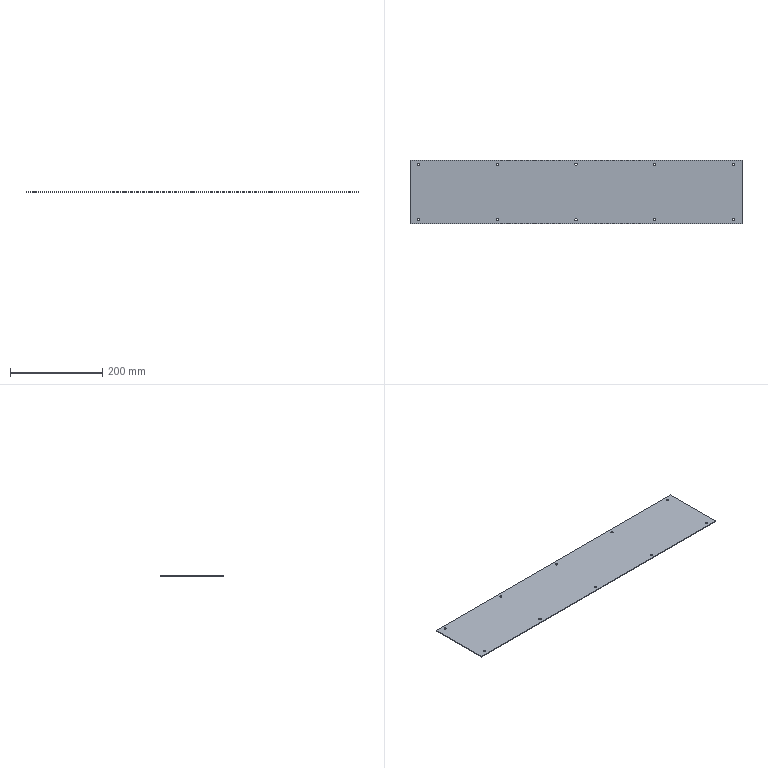Part | STEP file | 1 solid | 26 faces | box 718 x 138 x 1.5 mm | volume 148331 mm3 | cylinder 20 | plane 6 | commonest cylinder face diameters 5 x20